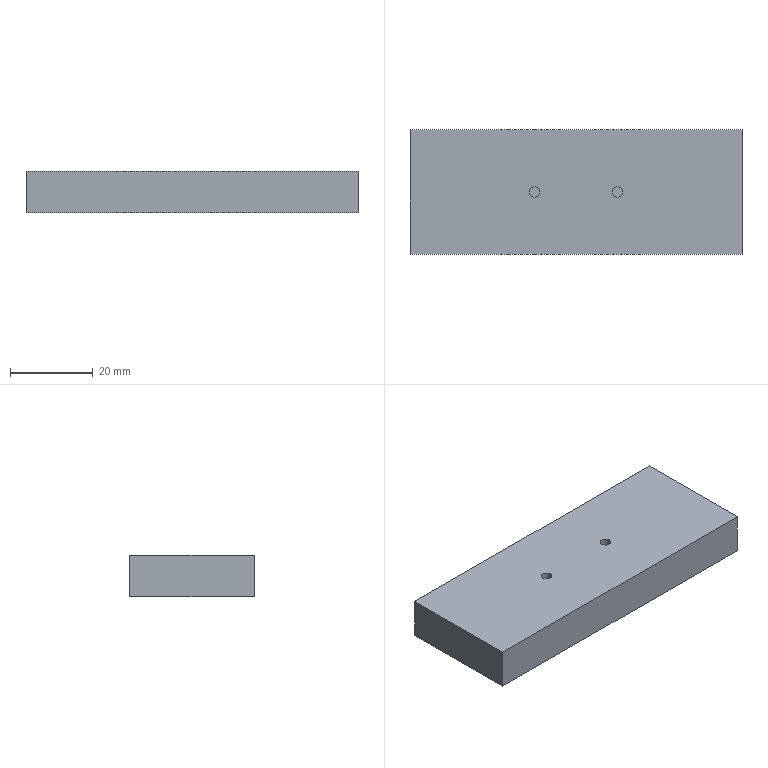Part | SolidWorks | features Extrusion 1, ICE 1 | 1 solid | 12 faces | box 80 x 30 x 10 mm | volume 23980 mm3 | plane 8 | cylinder 4 | commonest cylinder face diameters 2.5 x4
STEP:
#1=CARTESIAN_POINT('',(-11.25,0.,8.));
#2=VERTEX_POINT('',#1);
#3=CARTESIAN_POINT('',(-8.75,0.,8.));
#4=VERTEX_POINT('',#3);
#5=CARTESIAN_POINT('',(-10.,0.,8.));
#6=DIRECTION('',(0.,0.,1.));
#7=DIRECTION('',(1.,0.,0.));
#8=AXIS2_PLACEMENT_3D('',#5,#6,#7);
#9=CIRCLE('',#8,1.25);
#10=EDGE_CURVE('',#2,#4,#9,.T.);
#11=ORIENTED_EDGE('',*,*,#10,.F.);
#12=CARTESIAN_POINT('',(-11.25,0.,10.));
#13=VERTEX_POINT('',#12);
#14=CARTESIAN_POINT('',(-11.25,0.,8.));
#15=DIRECTION('',(0.,0.,1.));
#16=VECTOR('',#15,1000.);
#17=LINE('',#14,#16);
#18=EDGE_CURVE('',#2,#13,#17,.T.);
#19=ORIENTED_EDGE('',*,*,#18,.T.);
#20=CARTESIAN_POINT('',(-8.75,0.,10.));
#21=VERTEX_POINT('',#20);
#22=CARTESIAN_POINT('',(-10.,0.,10.));
#23=DIRECTION('',(0.,0.,1.));
#24=DIRECTION('',(1.,0.,0.));
#25=AXIS2_PLACEMENT_3D('',#22,#23,#24);
#26=CIRCLE('',#25,1.25);
#27=EDGE_CURVE('',#13,#21,#26,.T.);
#28=ORIENTED_EDGE('',*,*,#27,.T.);
#29=CARTESIAN_POINT('',(-8.75,0.,8.));
#30=DIRECTION('',(0.,0.,1.));
#31=VECTOR('',#30,1000.);
#32=LINE('',#29,#31);
#33=EDGE_CURVE('',#4,#21,#32,.T.);
#34=ORIENTED_EDGE('',*,*,#33,.F.);
#35=EDGE_LOOP('',(#11,#19,#28,#34));
#36=FACE_OUTER_BOUND('',#35,.T.);
#37=CARTESIAN_POINT('',(-10.,0.,8.));
#38=DIRECTION('',(0.,0.,1.));
#39=DIRECTION('',(1.,0.,0.));
#40=AXIS2_PLACEMENT_3D('',#37,#38,#39);
#41=CYLINDRICAL_SURFACE('',#40,1.25);
#42=ADVANCED_FACE('',(#36),#41,.F.);
#43=CARTESIAN_POINT('',(8.75,0.,8.));
#44=VERTEX_POINT('',#43);
#45=CARTESIAN_POINT('',(11.25,0.,8.));
#46=VERTEX_POINT('',#45);
#47=CARTESIAN_POINT('',(10.,0.,8.));
#48=DIRECTION('',(0.,0.,1.));
#49=DIRECTION('',(1.,0.,0.));
#50=AXIS2_PLACEMENT_3D('',#47,#48,#49);
#51=CIRCLE('',#50,1.25);
#52=EDGE_CURVE('',#44,#46,#51,.T.);
#53=ORIENTED_EDGE('',*,*,#52,.F.);
#54=CARTESIAN_POINT('',(8.75,0.,10.));
#55=VERTEX_POINT('',#54);
#56=CARTESIAN_POINT('',(8.75,0.,8.));
#57=DIRECTION('',(0.,0.,1.));
#58=VECTOR('',#57,1000.);
#59=LINE('',#56,#58);
#60=EDGE_CURVE('',#44,#55,#59,.T.);
#61=ORIENTED_EDGE('',*,*,#60,.T.);
#62=CARTESIAN_POINT('',(11.25,0.,10.));
#63=VERTEX_POINT('',#62);
#64=CARTESIAN_POINT('',(10.,0.,10.));
#65=DIRECTION('',(0.,0.,1.));
#66=DIRECTION('',(1.,0.,0.));
#67=AXIS2_PLACEMENT_3D('',#64,#65,#66);
#68=CIRCLE('',#67,1.25);
#69=EDGE_CURVE('',#55,#63,#68,.T.);
#70=ORIENTED_EDGE('',*,*,#69,.T.);
#71=CARTESIAN_POINT('',(11.25,0.,8.));
#72=DIRECTION('',(0.,0.,1.));
#73=VECTOR('',#72,1000.);
#74=LINE('',#71,#73);
#75=EDGE_CURVE('',#46,#63,#74,.T.);
#76=ORIENTED_EDGE('',*,*,#75,.F.);
#77=EDGE_LOOP('',(#53,#61,#70,#76));
#78=FACE_OUTER_BOUND('',#77,.T.);
#79=CARTESIAN_POINT('',(10.,0.,8.));
#80=DIRECTION('',(0.,0.,1.));
#81=DIRECTION('',(1.,0.,0.));
#82=AXIS2_PLACEMENT_3D('',#79,#80,#81);
#83=CYLINDRICAL_SURFACE('',#82,1.25);
#84=ADVANCED_FACE('',(#78),#83,.F.);
#85=CARTESIAN_POINT('',(-40.,15.,0.));
#86=VERTEX_POINT('',#85);
#87=CARTESIAN_POINT('',(-40.,-15.,0.));
#88=VERTEX_POINT('',#87);
#89=CARTESIAN_POINT('',(-40.,-15.,0.));
#90=DIRECTION('',(0.,-1.,0.));
#91=VECTOR('',#90,1000.);
#92=LINE('',#89,#91);
#93=EDGE_CURVE('',#86,#88,#92,.T.);
#94=ORIENTED_EDGE('',*,*,#93,.T.);
#95=CARTESIAN_POINT('',(-40.,-15.,10.));
#96=VERTEX_POINT('',#95);
#97=CARTESIAN_POINT('',(-40.,-15.,10.));
#98=DIRECTION('',(0.,0.,-1.));
#99=VECTOR('',#98,1000.);
#100=LINE('',#97,#99);
#101=EDGE_CURVE('',#96,#88,#100,.T.);
#102=ORIENTED_EDGE('',*,*,#101,.F.);
#103=CARTESIAN_POINT('',(-40.,15.,10.));
#104=VERTEX_POINT('',#103);
#105=CARTESIAN_POINT('',(-40.,-15.,10.));
#106=DIRECTION('',(0.,-1.,0.));
#107=VECTOR('',#106,1000.);
#108=LINE('',#105,#107);
#109=EDGE_CURVE('',#104,#96,#108,.T.);
#110=ORIENTED_EDGE('',*,*,#109,.F.);
#111=CARTESIAN_POINT('',(-40.,15.,10.));
#112=DIRECTION('',(0.,0.,-1.));
#113=VECTOR('',#112,1000.);
#114=LINE('',#111,#113);
#115=EDGE_CURVE('',#104,#86,#114,.T.);
#116=ORIENTED_EDGE('',*,*,#115,.T.);
#117=EDGE_LOOP('',(#94,#102,#110,#116));
#118=FACE_OUTER_BOUND('',#117,.T.);
#119=CARTESIAN_POINT('',(-40.,-15.,10.));
#120=DIRECTION('',(1.,0.,0.));
#121=DIRECTION('',(0.,0.,-1.));
#122=AXIS2_PLACEMENT_3D('',#119,#120,#121);
#123=PLANE('',#122);
#124=ADVANCED_FACE('',(#118),#123,.F.);
#125=CARTESIAN_POINT('',(40.,-15.,0.));
#126=VERTEX_POINT('',#125);
#127=CARTESIAN_POINT('',(40.,-15.,0.));
#128=DIRECTION('',(1.,0.,0.));
#129=VECTOR('',#128,1000.);
#130=LINE('',#127,#129);
#131=EDGE_CURVE('',#88,#126,#130,.T.);
#132=ORIENTED_EDGE('',*,*,#131,.T.);
#133=CARTESIAN_POINT('',(40.,-15.,10.));
#134=VERTEX_POINT('',#133);
#135=CARTESIAN_POINT('',(40.,-15.,10.));
#136=DIRECTION('',(0.,0.,-1.));
#137=VECTOR('',#136,1000.);
#138=LINE('',#135,#137);
#139=EDGE_CURVE('',#134,#126,#138,.T.);
#140=ORIENTED_EDGE('',*,*,#139,.F.);
#141=CARTESIAN_POINT('',(40.,-15.,10.));
#142=DIRECTION('',(1.,0.,0.));
#143=VECTOR('',#142,1000.);
#144=LINE('',#141,#143);
#145=EDGE_CURVE('',#96,#134,#144,.T.);
#146=ORIENTED_EDGE('',*,*,#145,.F.);
#147=ORIENTED_EDGE('',*,*,#101,.T.);
#148=EDGE_LOOP('',(#132,#140,#146,#147));
#149=FACE_OUTER_BOUND('',#148,.T.);
#150=CARTESIAN_POINT('',(40.,-15.,10.));
#151=DIRECTION('',(0.,1.,0.));
#152=DIRECTION('',(-1.,0.,0.));
#153=AXIS2_PLACEMENT_3D('',#150,#151,#152);
#154=PLANE('',#153);
#155=ADVANCED_FACE('',(#149),#154,.F.);
#156=CARTESIAN_POINT('',(40.,15.,0.));
#157=VERTEX_POINT('',#156);
#158=CARTESIAN_POINT('',(40.,-15.,0.));
#159=DIRECTION('',(0.,1.,0.));
#160=VECTOR('',#159,1000.);
#161=LINE('',#158,#160);
#162=EDGE_CURVE('',#126,#157,#161,.T.);
#163=ORIENTED_EDGE('',*,*,#162,.T.);
#164=CARTESIAN_POINT('',(40.,15.,10.));
#165=VERTEX_POINT('',#164);
#166=CARTESIAN_POINT('',(40.,15.,10.));
#167=DIRECTION('',(0.,0.,-1.));
#168=VECTOR('',#167,1000.);
#169=LINE('',#166,#168);
#170=EDGE_CURVE('',#165,#157,#169,.T.);
#171=ORIENTED_EDGE('',*,*,#170,.F.);
#172=CARTESIAN_POINT('',(40.,-15.,10.));
#173=DIRECTION('',(0.,1.,0.));
#174=VECTOR('',#173,1000.);
#175=LINE('',#172,#174);
#176=EDGE_CURVE('',#134,#165,#175,.T.);
#177=ORIENTED_EDGE('',*,*,#176,.F.);
#178=ORIENTED_EDGE('',*,*,#139,.T.);
#179=EDGE_LOOP('',(#163,#171,#177,#178));
#180=FACE_OUTER_BOUND('',#179,.T.);
#181=CARTESIAN_POINT('',(40.,-15.,10.));
#182=DIRECTION('',(-1.,0.,0.));
#183=DIRECTION('',(0.,0.,1.));
#184=AXIS2_PLACEMENT_3D('',#181,#182,#183);
#185=PLANE('',#184);
#186=ADVANCED_FACE('',(#180),#185,.F.);
#187=CARTESIAN_POINT('',(40.,15.,0.));
#188=DIRECTION('',(-1.,0.,0.));
#189=VECTOR('',#188,1000.);
#190=LINE('',#187,#189);
#191=EDGE_CURVE('',#157,#86,#190,.T.);
#192=ORIENTED_EDGE('',*,*,#191,.T.);
#193=ORIENTED_EDGE('',*,*,#115,.F.);
#194=CARTESIAN_POINT('',(40.,15.,10.));
#195=DIRECTION('',(-1.,0.,0.));
#196=VECTOR('',#195,1000.);
#197=LINE('',#194,#196);
#198=EDGE_CURVE('',#165,#104,#197,.T.);
#199=ORIENTED_EDGE('',*,*,#198,.F.);
#200=ORIENTED_EDGE('',*,*,#170,.T.);
#201=EDGE_LOOP('',(#192,#193,#199,#200));
#202=FACE_OUTER_BOUND('',#201,.T.);
#203=CARTESIAN_POINT('',(40.,15.,10.));
#204=DIRECTION('',(0.,-1.,0.));
#205=DIRECTION('',(1.,0.,0.));
#206=AXIS2_PLACEMENT_3D('',#203,#204,#205);
#207=PLANE('',#206);
#208=ADVANCED_FACE('',(#202),#207,.F.);
#209=CARTESIAN_POINT('',(-10.,0.,10.));
#210=DIRECTION('',(0.,0.,1.));
#211=DIRECTION('',(1.,0.,0.));
#212=AXIS2_PLACEMENT_3D('',#209,#210,#211);
#213=CIRCLE('',#212,1.25);
#214=EDGE_CURVE('',#21,#13,#213,.T.);
#215=ORIENTED_EDGE('',*,*,#214,.F.);
#216=ORIENTED_EDGE('',*,*,#27,.F.);
#217=EDGE_LOOP('',(#215,#216));
#218=FACE_BOUND('',#217,.T.);
#219=CARTESIAN_POINT('',(10.,0.,10.));
#220=DIRECTION('',(0.,0.,1.));
#221=DIRECTION('',(1.,0.,0.));
#222=AXIS2_PLACEMENT_3D('',#219,#220,#221);
#223=CIRCLE('',#222,1.25);
#224=EDGE_CURVE('',#63,#55,#223,.T.);
#225=ORIENTED_EDGE('',*,*,#224,.F.);
#226=ORIENTED_EDGE('',*,*,#69,.F.);
#227=EDGE_LOOP('',(#225,#226));
#228=FACE_BOUND('',#227,.T.);
#229=ORIENTED_EDGE('',*,*,#109,.T.);
#230=ORIENTED_EDGE('',*,*,#145,.T.);
#231=ORIENTED_EDGE('',*,*,#176,.T.);
#232=ORIENTED_EDGE('',*,*,#198,.T.);
#233=EDGE_LOOP('',(#229,#230,#231,#232));
#234=FACE_OUTER_BOUND('',#233,.T.);
#235=CARTESIAN_POINT('',(0.,0.,10.));
#236=DIRECTION('',(0.,0.,1.));
#237=DIRECTION('',(1.,0.,0.));
#238=AXIS2_PLACEMENT_3D('',#235,#236,#237);
#239=PLANE('',#238);
#240=ADVANCED_FACE('',(#218,#228,#234),#239,.T.);
#241=ORIENTED_EDGE('',*,*,#93,.F.);
#242=ORIENTED_EDGE('',*,*,#191,.F.);
#243=ORIENTED_EDGE('',*,*,#162,.F.);
#244=ORIENTED_EDGE('',*,*,#131,.F.);
#245=EDGE_LOOP('',(#241,#242,#243,#244));
#246=FACE_OUTER_BOUND('',#245,.T.);
#247=CARTESIAN_POINT('',(0.,0.,0.));
#248=DIRECTION('',(0.,0.,1.));
#249=DIRECTION('',(1.,0.,0.));
#250=AXIS2_PLACEMENT_3D('',#247,#248,#249);
#251=PLANE('',#250);
#252=ADVANCED_FACE('',(#246),#251,.F.);
#253=ORIENTED_EDGE('',*,*,#60,.F.);
#254=CARTESIAN_POINT('',(10.,0.,8.));
#255=DIRECTION('',(0.,0.,1.));
#256=DIRECTION('',(1.,0.,0.));
#257=AXIS2_PLACEMENT_3D('',#254,#255,#256);
#258=CIRCLE('',#257,1.25);
#259=EDGE_CURVE('',#46,#44,#258,.T.);
#260=ORIENTED_EDGE('',*,*,#259,.F.);
#261=ORIENTED_EDGE('',*,*,#75,.T.);
#262=ORIENTED_EDGE('',*,*,#224,.T.);
#263=EDGE_LOOP('',(#253,#260,#261,#262));
#264=FACE_OUTER_BOUND('',#263,.T.);
#265=CARTESIAN_POINT('',(10.,0.,8.));
#266=DIRECTION('',(0.,0.,1.));
#267=DIRECTION('',(1.,0.,0.));
#268=AXIS2_PLACEMENT_3D('',#265,#266,#267);
#269=CYLINDRICAL_SURFACE('',#268,1.25);
#270=ADVANCED_FACE('',(#264),#269,.F.);
#271=ORIENTED_EDGE('',*,*,#259,.T.);
#272=ORIENTED_EDGE('',*,*,#52,.T.);
#273=EDGE_LOOP('',(#271,#272));
#274=FACE_OUTER_BOUND('',#273,.T.);
#275=CARTESIAN_POINT('',(10.,0.,8.));
#276=DIRECTION('',(0.,0.,1.));
#277=DIRECTION('',(1.,0.,0.));
#278=AXIS2_PLACEMENT_3D('',#275,#276,#277);
#279=PLANE('',#278);
#280=ADVANCED_FACE('',(#274),#279,.T.);
#281=ORIENTED_EDGE('',*,*,#18,.F.);
#282=CARTESIAN_POINT('',(-10.,0.,8.));
#283=DIRECTION('',(0.,0.,1.));
#284=DIRECTION('',(1.,0.,0.));
#285=AXIS2_PLACEMENT_3D('',#282,#283,#284);
#286=CIRCLE('',#285,1.25);
#287=EDGE_CURVE('',#4,#2,#286,.T.);
#288=ORIENTED_EDGE('',*,*,#287,.F.);
#289=ORIENTED_EDGE('',*,*,#33,.T.);
#290=ORIENTED_EDGE('',*,*,#214,.T.);
#291=EDGE_LOOP('',(#281,#288,#289,#290));
#292=FACE_OUTER_BOUND('',#291,.T.);
#293=CARTESIAN_POINT('',(-10.,0.,8.));
#294=DIRECTION('',(0.,0.,1.));
#295=DIRECTION('',(1.,0.,0.));
#296=AXIS2_PLACEMENT_3D('',#293,#294,#295);
#297=CYLINDRICAL_SURFACE('',#296,1.25);
#298=ADVANCED_FACE('',(#292),#297,.F.);
#299=ORIENTED_EDGE('',*,*,#287,.T.);
#300=ORIENTED_EDGE('',*,*,#10,.T.);
#301=EDGE_LOOP('',(#299,#300));
#302=FACE_OUTER_BOUND('',#301,.T.);
#303=CARTESIAN_POINT('',(-10.,0.,8.));
#304=DIRECTION('',(0.,0.,1.));
#305=DIRECTION('',(1.,0.,0.));
#306=AXIS2_PLACEMENT_3D('',#303,#304,#305);
#307=PLANE('',#306);
#308=ADVANCED_FACE('',(#302),#307,.T.);
#309=CLOSED_SHELL('',(#42,#84,#124,#155,#186,#208,#240,#252,#270,#280,#298,#308));
#310=MANIFOLD_SOLID_BREP('',#309);
#311=CARTESIAN_POINT('',(0.,0.,0.));
#312=DIRECTION('',(0.,0.,1.));
#313=DIRECTION('',(1.,0.,0.));
#314=AXIS2_PLACEMENT_3D('',#311,#312,#313);
#315=(LENGTH_UNIT()NAMED_UNIT(*)SI_UNIT(.MILLI.,.METRE.));
#316=UNCERTAINTY_MEASURE_WITH_UNIT(LENGTH_MEASURE(0.00001),#315,'','');
#317=(NAMED_UNIT(*)PLANE_ANGLE_UNIT()SI_UNIT($,.RADIAN.));
#318=(NAMED_UNIT(*)SI_UNIT($,.STERADIAN.)SOLID_ANGLE_UNIT());
#319=(GEOMETRIC_REPRESENTATION_CONTEXT(3)GLOBAL_UNCERTAINTY_ASSIGNED_CONTEXT((#316))GLOBAL_UNIT_ASSIGNED_CONTEXT((#315,#317,#318))REPRESENTATION_CONTEXT('',''));
#320=ADVANCED_BREP_SHAPE_REPRESENTATION('',(#310,#314),#319);